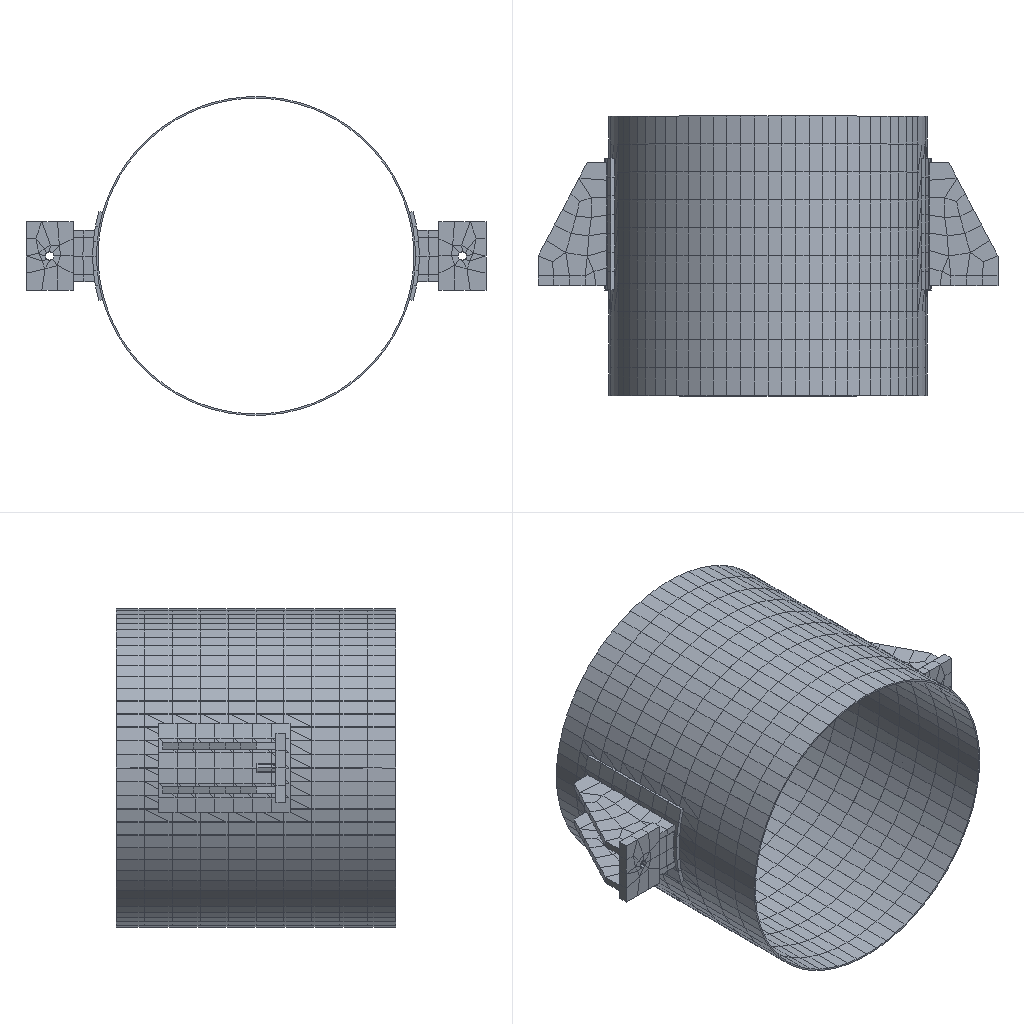Simulation study | ansys workbench
Ansys APDL input file, long lists of numbers shortened:
/batch
/config,noeldb,1     ! force off writing results to database
*get,_wallstrt,active,,time,wall
! ANSYS input file written by Workbench version 2022 R1
! File used for geometry attach:
/title,wbnew--____ (D5)
! ****** Begin Custom Load Command Snippet ******
/COM, ACT Extensions:
/COM,     LSDYNA, 2021.1
/COM,
! ****** End   Custom Load Command Snippet ******
*DIM,_wb_ProjectScratch_dir,string,248
_wb_ProjectScratch_dir(1) = ''
*DIM,_wb_SolverFiles_dir,string,248
_wb_SolverFiles_dir(1) = ''
*DIM,_wb_userfiles_dir,string,248
_wb_userfiles_dir(1) = ''
/com,--- Data in consistent NMM units. See Solving Units in the help system for more information.
/units,MPA
/nopr
/wb,file,start              !  signify a WB generated input file
/prep7
! Turn off shape checking because checks already performed inside WB mesher.
! See help system for more information.
SHPP,OFF,,NOWARN
/nolist
etcon,set             ! allow ANSYS to choose best KEYOP's for 180x elements, resets any applicable keyopt to MAPDL defaults
/com,*********** Nodes for the whole assembly ***********
nblock,3,,8465
(1i9,3e20.9e3)
        1     6.998606143E+01     1.422000000E+03     7.999443426E+02
! (7695 more lines like these left out)
-1
/wb,elem,start            !  set before creation of elements
/com,*********** Elements for Body 1 "__1^___1|__-__1" ***********
et,1,186
keyo,1,2,1          ! set full integration on SOLID186
eblock,19,solid,,720
(19i9)
        1        1        1        1        0        0        0        0       20        0        1      458     1166     1165      459      462     1201     1200      460
! (1439 more lines like these left out)
-1
/com,*********** Elements for Body 2 "__2^___1|__-__1" ***********
et,2,186
keyo,2,2,1          ! set full integration on SOLID186
eblock,19,solid,,42
(19i9)
        2        2        2        2        0        0        0        0       20        0      721     5444     5464     5493     5499     5455     5456     5492     5512
! (83 more lines like these left out)
-1
/com,*********** Elements for Body 3 "__3^___1|__-__1" ***********
et,3,186
keyo,3,2,1          ! set full integration on SOLID186
eblock,19,solid,,21
(19i9)
        3        3        3        3        0        0        0        0       20        0      763     5764     5813     5769     5765     5779     5791     5774     5778
! (41 more lines like these left out)
-1
/com,*********** Elements for Body 4 "__4^___1|__-__1" ***********
et,4,186
keyo,4,2,1          ! set full integration on SOLID186
eblock,19,solid,,20
(19i9)
        4        4        4        4        0        0        0        0       20        0      784     5965     5966     5967     5968     5974     5973     5972     5971
! (39 more lines like these left out)
-1
/com,*********** Elements for Body 5 "__4^___1|__-__1[2]" ***********
et,5,186
keyo,5,2,1          ! set full integration on SOLID186
eblock,19,solid,,20
(19i9)
        5        5        5        5        0        0        0        0       20        0      804     6158     6159     6160     6161     6167     6166     6165     6164
! (39 more lines like these left out)
-1
! (8 more sections like these left out)
/wb,elem,end               !  done creating elements
/com,*********** Send User Defined Coordinate System(s) ***********
csys,0
toffst,273.15,  ! Temperature offset from absolute zero
/com,*********** Set Reference Temperature ***********
tref,22.
/wb,mat,start              !  starting to send materials
/com,*********** Send Materials ***********
Temperature = 'TEMP' ! Temperature
MP,DENS,1,7.85e-09,	! tonne mm^-3
MP,ALPX,1,1.2e-05,	! C^-1
MP,C,1,434000000,	! mm^2 s^-2 C^-1
MP,KXX,1,60.5,	! tonne mm s^-3 C^-1
MP,RSVX,1,0.00017,	! ohm mm
MP,EX,1,200000,	! tonne s^-2 mm^-1
MP,NUXY,1,0.3,
MP,MURX,1,10000,
Temperature = 'TEMP' ! Temperature
MP,DENS,2,7.85e-09,	! tonne mm^-3
MP,ALPX,2,1.2e-05,	! C^-1
MP,C,2,434000000,	! mm^2 s^-2 C^-1
MP,KXX,2,60.5,	! tonne mm s^-3 C^-1
MP,RSVX,2,0.00017,	! ohm mm
MP,EX,2,200000,	! tonne s^-2 mm^-1
MP,NUXY,2,0.3,
MP,MURX,2,10000,
Temperature = 'TEMP' ! Temperature
MP,DENS,3,7.85e-09,	! tonne mm^-3
MP,ALPX,3,1.2e-05,	! C^-1
MP,C,3,434000000,	! mm^2 s^-2 C^-1
MP,KXX,3,60.5,	! tonne mm s^-3 C^-1
MP,RSVX,3,0.00017,	! ohm mm
MP,EX,3,200000,	! tonne s^-2 mm^-1
MP,NUXY,3,0.3,
MP,MURX,3,10000,
Temperature = 'TEMP' ! Temperature
MP,DENS,4,7.85e-09,	! tonne mm^-3
MP,ALPX,4,1.2e-05,	! C^-1
MP,C,4,434000000,	! mm^2 s^-2 C^-1
MP,KXX,4,60.5,	! tonne mm s^-3 C^-1
MP,RSVX,4,0.00017,	! ohm mm
MP,EX,4,200000,	! tonne s^-2 mm^-1
MP,NUXY,4,0.3,
MP,MURX,4,10000,
Temperature = 'TEMP' ! Temperature
MP,DENS,5,7.85e-09,	! tonne mm^-3
MP,ALPX,5,1.2e-05,	! C^-1
MP,C,5,434000000,	! mm^2 s^-2 C^-1
MP,KXX,5,60.5,	! tonne mm s^-3 C^-1
MP,RSVX,5,0.00017,	! ohm mm
MP,EX,5,200000,	! tonne s^-2 mm^-1
MP,NUXY,5,0.3,
MP,MURX,5,10000,
Temperature = 'TEMP' ! Temperature
MP,DENS,6,7.85e-09,	! tonne mm^-3
MP,ALPX,6,1.2e-05,	! C^-1
MP,C,6,434000000,	! mm^2 s^-2 C^-1
MP,KXX,6,60.5,	! tonne mm s^-3 C^-1
MP,RSVX,6,0.00017,	! ohm mm
MP,EX,6,200000,	! tonne s^-2 mm^-1
MP,NUXY,6,0.3,
MP,MURX,6,10000,
Temperature = 'TEMP' ! Temperature
MP,DENS,7,7.85e-09,	! tonne mm^-3
MP,ALPX,7,1.2e-05,	! C^-1
MP,C,7,434000000,	! mm^2 s^-2 C^-1
MP,KXX,7,60.5,	! tonne mm s^-3 C^-1
MP,RSVX,7,0.00017,	! ohm mm
MP,EX,7,200000,	! tonne s^-2 mm^-1
MP,NUXY,7,0.3,
MP,MURX,7,10000,
Temperature = 'TEMP' ! Temperature
MP,DENS,8,7.85e-09,	! tonne mm^-3
MP,ALPX,8,1.2e-05,	! C^-1
MP,C,8,434000000,	! mm^2 s^-2 C^-1
MP,KXX,8,60.5,	! tonne mm s^-3 C^-1
MP,RSVX,8,0.00017,	! ohm mm
MP,EX,8,200000,	! tonne s^-2 mm^-1
MP,NUXY,8,0.3,
MP,MURX,8,10000,
Temperature = 'TEMP' ! Temperature
MP,DENS,9,7.85e-09,	! tonne mm^-3
MP,ALPX,9,1.2e-05,	! C^-1
MP,C,9,434000000,	! mm^2 s^-2 C^-1
MP,KXX,9,60.5,	! tonne mm s^-3 C^-1
MP,RSVX,9,0.00017,	! ohm mm
MP,EX,9,200000,	! tonne s^-2 mm^-1
MP,NUXY,9,0.3,
MP,MURX,9,10000,
Temperature = 'TEMP' ! Temperature
MP,DENS,10,7.85e-09,	! tonne mm^-3
MP,ALPX,10,1.2e-05,	! C^-1
MP,C,10,434000000,	! mm^2 s^-2 C^-1
MP,KXX,10,60.5,	! tonne mm s^-3 C^-1
MP,RSVX,10,0.00017,	! ohm mm
MP,EX,10,200000,	! tonne s^-2 mm^-1
MP,NUXY,10,0.3,
MP,MURX,10,10000,
Temperature = 'TEMP' ! Temperature
MP,DENS,11,7.85e-09,	! tonne mm^-3
MP,ALPX,11,1.2e-05,	! C^-1
MP,C,11,434000000,	! mm^2 s^-2 C^-1
MP,KXX,11,60.5,	! tonne mm s^-3 C^-1
MP,RSVX,11,0.00017,	! ohm mm
MP,EX,11,200000,	! tonne s^-2 mm^-1
MP,NUXY,11,0.3,
MP,MURX,11,10000,
Temperature = 'TEMP' ! Temperature
MP,DENS,12,7.85e-09,	! tonne mm^-3
MP,ALPX,12,1.2e-05,	! C^-1
MP,C,12,434000000,	! mm^2 s^-2 C^-1
MP,KXX,12,60.5,	! tonne mm s^-3 C^-1
MP,RSVX,12,0.00017,	! ohm mm
MP,EX,12,200000,	! tonne s^-2 mm^-1
MP,NUXY,12,0.3,
MP,MURX,12,10000,
Temperature = 'TEMP' ! Temperature
MP,DENS,13,7.85e-09,	! tonne mm^-3
MP,ALPX,13,1.2e-05,	! C^-1
MP,C,13,434000000,	! mm^2 s^-2 C^-1
MP,KXX,13,60.5,	! tonne mm s^-3 C^-1
MP,RSVX,13,0.00017,	! ohm mm
MP,EX,13,200000,	! tonne s^-2 mm^-1
MP,NUXY,13,0.3,
MP,MURX,13,10000,
/wb,mat,end                !  done sending materials
!************************* Model Summary ********************
!__1^___1|__-__1,	Q355E,	matid,	1
!__2^___1|__-__1,	Q355E,	matid,	2
!__3^___1|__-__1,	Q355E,	matid,	3
!__4^___1|__-__1,	Q355E,	matid,	4
!__4^___1|__-__1[2],	Q355E,	matid,	5
!__5^___1|__-__1,	Q355E,	matid,	6
!__2^___1|__-__1[2],	Q355E,	matid,	7
!__4^___1|__-__1[3],	Q355E,	matid,	8
!__4^___1|__-__1[4],	Q355E,	matid,	9
!__3^___1|__-__1[2],	Q355E,	matid,	10
!__5^___1|__-__1[2],	Q355E,	matid,	11
!__6^___1|__-__1,	Q355E,	matid,	12
!__6^___1|__-__1[2],	Q355E,	matid,	13
!************************* End Model Summary ********************
! get the diagonal of the bounding box. Needed later for other things
*get,_xmin,node,,mnloc,x
*get,_ymin,node,,mnloc,y
*get,_zmin,node,,mnloc,z
*get,_xmax,node,,mxloc,x
*get,_ymax,node,,mxloc,y
*get,_zmax,node,,mxloc,z
_ASMDIAG=(_xmax-_xmin)*(_xmax-_xmin)+(_ymax-_ymin)*(_ymax-_ymin)+(_zmax-_zmin)*(_zmax-_zmin)
_ASMDIAG=SQRT(_ASMDIAG)
/wb,contact,start          !  starting to send contact
/com,*********** Create Contact "接触区域" ***********
/com,            Real Constant Set For Above Contact Is 15 & 14
*set,tid,15
*set,cid,14
r,tid
r,cid
et,tid,170
et,cid,174
eblock,10,,,48
(15i9)
     3271       15       15       15        0      563      564      529      528     3174     3072     3068     3069
! (47 more lines like these left out)
-1
eblock,10,,,48
(15i9)
     3319       14       14       14        0      563      564      529      528     3174     3072     3068     3069
! (47 more lines like these left out)
-1
eblock,10,,,42
(15i9)
     3367       14       15       14        0     5465     5443     5457     5458     5629     5628     5673     5675
! (41 more lines like these left out)
-1
eblock,10,,,42
(15i9)
     3409       15       14       15        0     5465     5443     5457     5458     5629     5628     5673     5675
! (41 more lines like these left out)
-1
keyo,cid,8,2               ! auto create asymmetric contact (from Program Controlled setting)
keyo,cid,10,0              ! adjust contact stiffness each NR iteration (from Program Controlled setting)
keyo,cid,12,5              ! bonded always
keyo,cid,18,1              ! small sliding turned on by application
keyo,cid,2,0               ! augmented Lagrange (from Program Controlled setting)
keyo,cid,4,0               ! on Gauss point (from Program Controlled setting)
keyo,cid,9,1               ! ignore initial gaps/penetration
keyo,cid,7,0               ! No Prediction
rmod,tid,3,10.      ! FKN
rmod,tid,5,0.       ! ICONT
rmod,tid,6,0.       ! PINB
rmod,tid,10,0.      ! CNOF
rmod,tid,12,0.      ! FKT
rmod,tid,36,56      ! WB DSID
rmod,cid,3,10.      ! FKN
rmod,cid,5,0.       ! ICONT
rmod,cid,6,0.       ! PINB
rmod,cid,10,0.      ! CNOF
rmod,cid,12,0.      ! FKT
rmod,cid,36,56      ! WB DSID
/com,*********** Create Contact "接触区域 2" ***********
/com,            Real Constant Set For Above Contact Is 17 & 16
*set,tid,17
*set,cid,16
r,tid
r,cid
et,tid,170
et,cid,174
eblock,10,,,48
(15i9)
     3451       17       17       17        0      933      934      899      898     4186     4120     4117     4118
! (47 more lines like these left out)
-1
eblock,10,,,48
(15i9)
     3499       16       16       16        0      933      934      899      898     4186     4120     4117     4118
! (47 more lines like these left out)
-1
eblock,10,,,42
(15i9)
     3547       16       17       16        0     6461     6439     6453     6454     6625     6624     6669     6671
! (41 more lines like these left out)
-1
eblock,10,,,42
(15i9)
     3589       17       16       17        0     6461     6439     6453     6454     6625     6624     6669     6671
! (41 more lines like these left out)
-1
keyo,cid,8,2               ! auto create asymmetric contact (from Program Controlled setting)
keyo,cid,10,0              ! adjust contact stiffness each NR iteration (from Program Controlled setting)
keyo,cid,12,5              ! bonded always
keyo,cid,18,1              ! small sliding turned on by application
keyo,cid,2,0               ! augmented Lagrange (from Program Controlled setting)
keyo,cid,4,0               ! on Gauss point (from Program Controlled setting)
keyo,cid,9,1               ! ignore initial gaps/penetration
keyo,cid,7,0               ! No Prediction
rmod,tid,3,10.      ! FKN
rmod,tid,5,0.       ! ICONT
rmod,tid,6,0.       ! PINB
rmod,tid,10,0.      ! CNOF
rmod,tid,12,0.      ! FKT
rmod,tid,36,59      ! WB DSID
rmod,cid,3,10.      ! FKN
rmod,cid,5,0.       ! ICONT
rmod,cid,6,0.       ! PINB
rmod,cid,10,0.      ! CNOF
rmod,cid,12,0.      ! FKT
rmod,cid,36,59      ! WB DSID
/com,*********** Create Contact "接触区域 3" ***********
/com,            Real Constant Set For Above Contact Is 19 & 18
*set,tid,19
*set,cid,18
r,tid
r,cid
et,tid,170
et,cid,174
eblock,10,,,7
(15i9)
     3631       19       19       19        0     5415     5416     5427     5429     5546     5552     5589     5548
! (6 more lines like these left out)
-1
eblock,10,,,7
(15i9)
     3638       18       18       18        0     5415     5416     5427     5429     5546     5552     5589     5548
! (6 more lines like these left out)
-1
eblock,10,,,7
(15i9)
     3645       18       19       18        0     6015     6016     5985     5986     6147     6101     6099     6103
! (6 more lines like these left out)
-1
eblock,10,,,7
(15i9)
     3652       19       18       19        0     6015     6016     5985     5986     6147     6101     6099     6103
! (6 more lines like these left out)
-1
keyo,cid,8,2               ! auto create asymmetric contact (from Program Controlled setting)
keyo,cid,10,0              ! adjust contact stiffness each NR iteration (from Program Controlled setting)
keyo,cid,12,5              ! bonded always
keyo,cid,18,1              ! small sliding turned on by application
keyo,cid,2,0               ! augmented Lagrange (from Program Controlled setting)
keyo,cid,4,0               ! on Gauss point (from Program Controlled setting)
keyo,cid,9,1               ! ignore initial gaps/penetration
keyo,cid,7,0               ! No Prediction
rmod,tid,3,10.      ! FKN
rmod,tid,5,0.       ! ICONT
rmod,tid,6,0.       ! PINB
rmod,tid,10,0.      ! CNOF
rmod,tid,12,0.      ! FKT
rmod,tid,36,62      ! WB DSID
rmod,cid,3,10.      ! FKN
rmod,cid,5,0.       ! ICONT
rmod,cid,6,0.       ! PINB
rmod,cid,10,0.      ! CNOF
rmod,cid,12,0.      ! FKT
rmod,cid,36,62      ! WB DSID
/com,*********** Create Contact "接触区域 4" ***********
/com,            Real Constant Set For Above Contact Is 21 & 20
*set,tid,21
*set,cid,20
r,tid
r,cid
et,tid,170
et,cid,174
eblock,10,,,7
(15i9)
     3659       21       21       21        0     5499     5500     5511     5512     5744     5748     5762     5746
! (6 more lines like these left out)
-1
eblock,10,,,7
(15i9)
     3666       20       20       20        0     5499     5500     5511     5512     5744     5748     5762     5746
! (6 more lines like these left out)
-1
eblock,10,,,7
(15i9)
     3673       20       21       20        0     6208     6209     6178     6179     6340     6294     6292     6296
! (6 more lines like these left out)
-1
eblock,10,,,7
(15i9)
     3680       21       20       21        0     6208     6209     6178     6179     6340     6294     6292     6296
! (6 more lines like these left out)
-1
keyo,cid,8,2               ! auto create asymmetric contact (from Program Controlled setting)
keyo,cid,10,0              ! adjust contact stiffness each NR iteration (from Program Controlled setting)
keyo,cid,12,5              ! bonded always
keyo,cid,18,1              ! small sliding turned on by application
keyo,cid,2,0               ! augmented Lagrange (from Program Controlled setting)
keyo,cid,4,0               ! on Gauss point (from Program Controlled setting)
keyo,cid,9,1               ! ignore initial gaps/penetration
keyo,cid,7,0               ! No Prediction
rmod,tid,3,10.      ! FKN
rmod,tid,5,0.       ! ICONT
rmod,tid,6,0.       ! PINB
rmod,tid,10,0.      ! CNOF
rmod,tid,12,0.      ! FKT
rmod,tid,36,65      ! WB DSID
rmod,cid,3,10.      ! FKN
rmod,cid,5,0.       ! ICONT
rmod,cid,6,0.       ! PINB
rmod,cid,10,0.      ! CNOF
rmod,cid,12,0.      ! FKT
rmod,cid,36,65      ! WB DSID
/com,*********** Create Contact "接触区域 5" ***********
/com,            Real Constant Set For Above Contact Is 23 & 22
*set,tid,23
*set,cid,22
r,tid
r,cid
et,tid,170
et,cid,174
eblock,10,,,4
(15i9)
     3687       23       23       23        0     5437     5415     5429     5430     5549     5548     5593     5595
     3688       23       23       23        0     5415     5416     5427     5429     5546     5552     5589     5548
     3689       23       23       23        0     5499     5500     5511     5512     5744     5748     5762     5746
     3690       23       23       23        0     5500     5437     5430     5511     5611     5595     5597     5748
-1
eblock,10,,,4
(15i9)
     3691       22       22       22        0     5437     5415     5429     5430     5549     5548     5593     5595
     3692       22       22       22        0     5415     5416     5427     5429     5546     5552     5589     5548
     3693       22       22       22        0     5499     5500     5511     5512     5744     5748     5762     5746
     3694       22       22       22        0     5500     5437     5430     5511     5611     5595     5597     5748
-1
eblock,10,,,2
(15i9)
     3695       22       23       22        0     6359     6356     6354     6353     6390     6387     6384     6385
     3696       22       23       22        0     6356     6357     6355     6354     6389     6388     6386     6387
-1
eblock,10,,,2
(15i9)
     3697       23       22       23        0     6359     6356     6354     6353     6390     6387     6384     6385
     3698       23       22       23        0     6356     6357     6355     6354     6389     6388     6386     6387
-1
keyo,cid,8,2               ! auto create asymmetric contact (from Program Controlled setting)
keyo,cid,10,0              ! adjust contact stiffness each NR iteration (from Program Controlled setting)
keyo,cid,12,5              ! bonded always
keyo,cid,18,1              ! small sliding turned on by application
keyo,cid,2,0               ! augmented Lagrange (from Program Controlled setting)
keyo,cid,4,0               ! on Gauss point (from Program Controlled setting)
keyo,cid,9,1               ! ignore initial gaps/penetration
keyo,cid,7,0               ! No Prediction
rmod,tid,3,10.      ! FKN
rmod,tid,5,0.       ! ICONT
rmod,tid,6,0.       ! PINB
rmod,tid,10,0.      ! CNOF
rmod,tid,12,0.      ! FKT
rmod,tid,36,68      ! WB DSID
rmod,cid,3,10.      ! FKN
rmod,cid,5,0.       ! ICONT
rmod,cid,6,0.       ! PINB
rmod,cid,10,0.      ! CNOF
rmod,cid,12,0.      ! FKT
rmod,cid,36,68      ! WB DSID
! (15 more sections like these left out)
/wb,contact,end            !  done creating contacts
/com,*********** Send Named Selection as Node Component ***********
CMBLOCK,______  ,NODE,      208
(8i10)
      5781      5782      5783      5798      5799      5800      5801      5802
! (25 more lines like these left out)
/golist
/wb,load,start             !  starting to send loads
/com,*********** Fixed Supports ***********
CMBLOCK,_FIXEDSU,NODE,      208
(8i10)
      5781      5782      5783      5798      5799      5800      5801      5802
! (25 more lines like these left out)
cmsel,s,_FIXEDSU
d,all,all
nsel,all
/com,*********** Define Force Using Surface Effect Elements ***********
local,12,0,0.,0.,0.,0.,0.,0.
csys,0
et,54,154
eblock,10,,,42
(15i9)
     3999       54       54       54       12     7160     7156     7159     7159     7256     7255     7159     7265
! (41 more lines like these left out)
-1
esel,s,type,,54
keyop,54,2,1                ! Apply load in local coordinate system
keyop,54,7,1                ! Use original area so load is constant in large deformation
esel,all
/gst,on,on
fini
*get,_numnode,node,0,count
*get,_numelem,elem,0,count
*get, _MAXELEMNUM, elem, 0, NUM, MAX
*get, _MAXNODENUM, node, 0, NUM, MAX
*get, _MAXELEMTYPE, etyp, 0, NUM, MAX
*get, _MAXREALCONST, real, 0, NUM, MAX
/go
/wb,load,end               !  done creating loads
/com,--- Number of total nodes = %_numnode%
/com,--- Number of contact elements = 770
/com,--- Number of spring elements = 0
/com,--- Number of bearing elements = 0
/com,--- Number of solid elements = 966
/com,--- Number of condensed parts = 0
/com,--- Number of total elements = %_numelem%
*get,_wallbsol,active,,time,wall
/com,****************************************************************************
/com,*************************    SOLUTION       ********************************
/com,****************************************************************************
/solu
antype,0                   ! static analysis
_thickRatio=  0     ! Ratio of thick parts in the model
eqsl,sparse,,,,,1
cntr,print,1               ! print out contact info and also make no initial contact an error
dmpoption,emat,no             ! Don't combine emat file for DANSYS
dmpoption,esav,no             ! Don't combine esav file for DANSYS
nldiag,cont,iter           ! print out contact info each equilibrium iteration
rescontrol,,none                 ! Do not keep any restart files
/com,****************************************************
/com,******************* SOLVE FOR LS 1 OF 1 ****************
esel,s,type,,54
nsle
sfe,all,1,pres,1,0.
sfe,all,2,pres,1,3.65
sfe,all,3,pres,1,0.
nsel,all
esel,all
/nopr
/gopr
nsub,1,1,1
time,1.
outres,erase
outres,all,none
outres,nsol,all,
outres,rsol,all
outres,eangl,all
outres,etmp,all
outres,veng,all
outres,strs,all,
outres,epel,all,
outres,eppl,all,
outres,cont,all,
! *********** WB SOLVE COMMAND ***********
! check interactive state
*get,ANSINTER_,active,,int
*if,ANSINTER_,ne,0,then
/eof
*endif
solve
/com *************** Write FE CONNECTORS *********
CEWRITE,file,ce,,INTE
/com,****************************************************
/com,*************** FINISHED SOLVE FOR LS 1 *************
*get,_wallasol,active,,time,wall
/nopr
*get,_numnode,node,0,count
*get,_numelem,elem,0,count
*get, _MAXELEMNUM, elem, 0, NUM, MAX
*get, _MAXNODENUM, node, 0, NUM, MAX,,,INTERNAL
*get, _MAXELEMTYPE, etyp, 0, NUM, MAX
*get, _MAXREALCONST, real, 0, NUM, MAX
/gopr
/post1
xmlo,ENCODING,ISO-8859-1
xmlo,parm
/xml,parm,xml
fini
/gopr
*get,_walldone,active,,time,wall
_preptime=(_wallbsol-_wallstrt)*3600
_solvtime=(_wallasol-_wallbsol)*3600
_posttime=(_walldone-_wallasol)*3600
_totaltim=(_walldone-_wallstrt)*3600
*get,_dlbratio,active,0,solu,dlbr
*get,_combtime,active,0,solu,comb
*get,_ssmode,active,0,solu,ssmm
*get,_ndofs,active,0,solu,ndof
*get,_sol_end_time,active,0,set,time
*if,_sol_end_time,eq,1.,then
/fclean				!clean distributed files
*endif
/com,--- Total number of nodes = %_numnode%
/com,--- Total number of elements = %_numelem%
/com,--- Element load balance ratio = %_dlbratio%
/com,--- Time to combine distributed files = %_combtime%
/com,--- Sparse memory mode = %_ssmode%
/com,--- Number of DOF = %_ndofs%
/wb,file,end               ! done with WB generated input